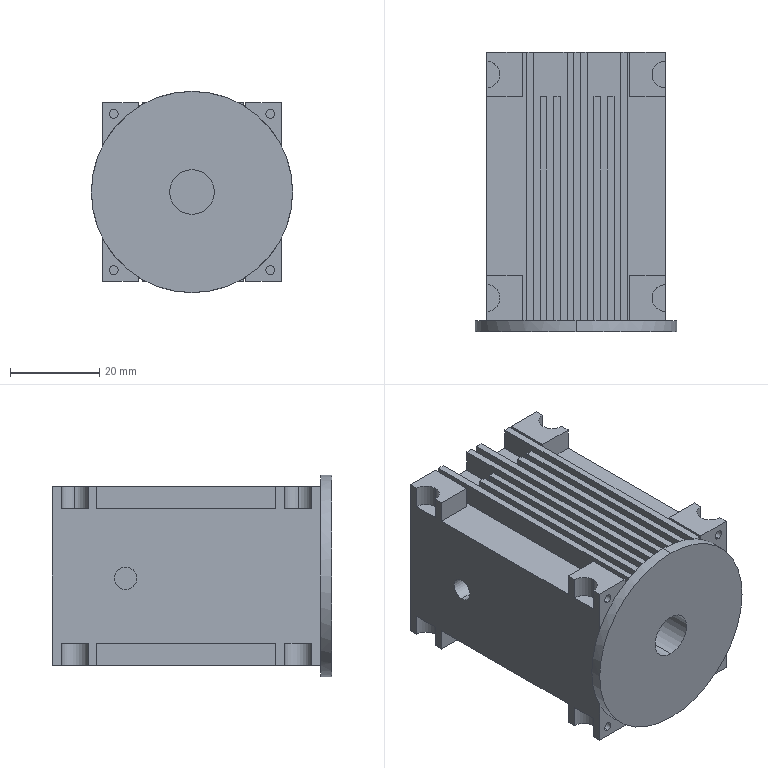Part | SolidWorks | features ICE 8, MirrorPattern 3, Extrusion 1 | 1 solid | 150 faces | box 45 x 62.5 x 45 mm | volume 83814 mm3 | plane 124 | cylinder 26 | commonest cylinder face diameters 6 x12 2 x8 5 x2 10 x2 45 x2